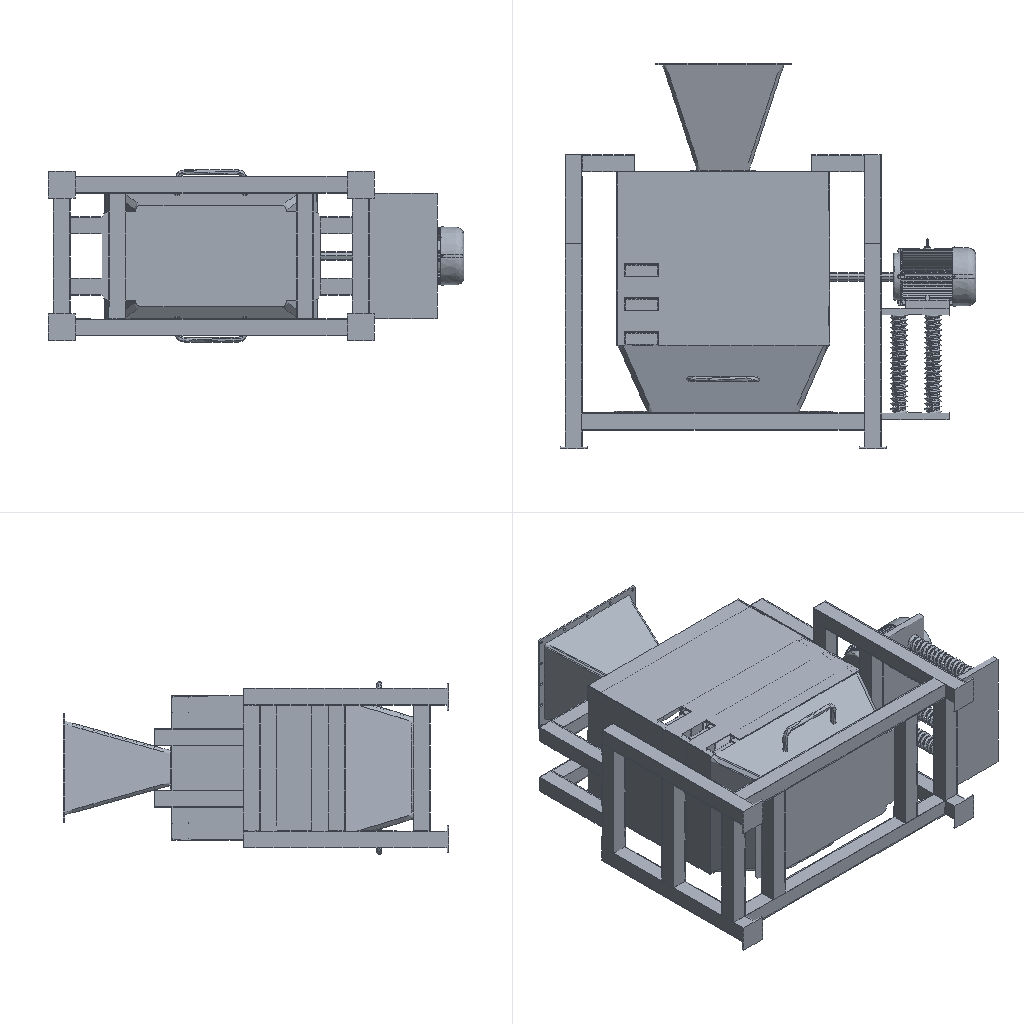Simulation study | ansys workbench
Set-up summary, first 221 of 611 lines:
category,name,step,type,value,unit,region
solver,ansys_mapdl
solver,version,,,21.2
solver,version,,,21.2
solver,version,,,21.2
solver,version,,,21.2
units,MPA,,stated
analysis,deck1,,modal,modal
load_step,requested,,,2
analysis,nlgeom,,,False
mesh,nodes,,,0
mesh,elements,,,0
load,load commands in deck,,count,0
bc,support commands in deck,,count,0
analysis,deck2,,static,static
load_step,requested,,,1
analysis,nlgeom,,,False
mesh,nodes,,,125678
mesh,elements,,,54949
element_type,ANSYS 187 (type 1),,solid,4190
element_type,ANSYS 186 (type 2),,solid,112
element_type,ANSYS 186 (type 3),,solid,154
element_type,ANSYS 186 (type 4),,solid,99
element_type,ANSYS 186 (type 5),,solid,109
element_type,ANSYS 186 (type 6),,solid,80
element_type,ANSYS 186 (type 7),,solid,144
element_type,ANSYS 186 (type 8),,solid,96
element_type,ANSYS 186 (type 9),,solid,96
element_type,ANSYS 186 (type 10),,solid,96
element_type,ANSYS 186 (type 11),,solid,132
element_type,ANSYS 186 (type 12),,solid,96
element_type,ANSYS 186 (type 13),,solid,132
element_type,ANSYS 187 (type 14),,solid,3160
element_type,ANSYS 186 (type 15),,solid,96
element_type,ANSYS 186 (type 16),,solid,96
element_type,ANSYS 186 (type 17),,solid,96
element_type,ANSYS 186 (type 18),,solid,88
element_type,ANSYS 186 (type 19),,solid,88
element_type,ANSYS 186 (type 20),,solid,88
element_type,ANSYS 186 (type 21),,solid,506
element_type,ANSYS 186 (type 22),,solid,80
element_type,ANSYS 186 (type 23),,solid,80
element_type,ANSYS 186 (type 24),,solid,80
element_type,ANSYS 186 (type 25),,solid,80
element_type,ANSYS 186 (type 26),,solid,80
element_type,ANSYS 187 (type 27),,solid,574
element_type,ANSYS 186 (type 28),,solid,45
element_type,ANSYS 186 (type 29),,solid,45
element_type,ANSYS 186 (type 30),,solid,20
element_type,ANSYS 186 (type 31),,solid,20
element_type,ANSYS 186 (type 32),,solid,20
element_type,ANSYS 186 (type 33),,solid,20
element_type,ANSYS 186 (type 34),,solid,20
element_type,ANSYS 186 (type 35),,solid,20
element_type,ANSYS 186 (type 36),,solid,160
element_type,ANSYS 186 (type 37),,solid,160
element_type,ANSYS 186 (type 38),,solid,160
element_type,ANSYS 186 (type 39),,solid,160
element_type,ANSYS 186 (type 40),,solid,160
element_type,ANSYS 186 (type 41),,solid,160
element_type,ANSYS 186 (type 42),,solid,160
element_type,ANSYS 186 (type 43),,solid,160
element_type,ANSYS 187 (type 44),,solid,19818
element_type,ANSYS 186 (type 45),,solid,144
element_type,ANSYS 186 (type 46),,solid,144
element_type,ANSYS 186 (type 47),,solid,144
element_type,ANSYS 186 (type 48),,solid,144
element_type,ANSYS 187 (type 49),,solid,1310
element_type,ANSYS 187 (type 50),,solid,1347
element_type,ANSYS 187 (type 51),,solid,1310
element_type,ANSYS 187 (type 52),,solid,1347
element_type,ANSYS 186 (type 53),,solid,128
element_type,ANSYS 186 (type 54),,solid,128
element_type,ANSYS 186 (type 55),,solid,128
element_type,ANSYS 186 (type 56),,solid,128
element_type,ANSYS 186 (type 57),,solid,192
element_type,ANSYS 186 (type 58),,solid,192
element_type,ANSYS 186 (type 59),,solid,192
element_type,ANSYS 186 (type 60),,solid,192
element_type,ANSYS 187 (type 61),,solid,1312
element_type,ANSYS 187 (type 62),,solid,1313
element_type,ANSYS 187 (type 63),,solid,1326
element_type,ANSYS 186 (type 64),,solid,36
element_type,ANSYS 186 (type 65),,solid,36
element_type,ANSYS 186 (type 66),,solid,36
element_type,ANSYS 186 (type 67),,solid,36
element_type,ANSYS 186 (type 68),,solid,56
element_type,ANSYS 186 (type 69),,solid,52
element_type,ANSYS 174 (type 70),,contact,70
element_type,ANSYS 170 (type 71),,target,70
element_type,ANSYS 174 (type 72),,contact,59
element_type,ANSYS 170 (type 73),,target,59
element_type,ANSYS 174 (type 74),,contact,64
element_type,ANSYS 170 (type 75),,target,64
element_type,ANSYS 174 (type 76),,contact,64
element_type,ANSYS 170 (type 77),,target,64
element_type,ANSYS 174 (type 78),,contact,254
element_type,ANSYS 170 (type 79),,target,254
element_type,ANSYS 174 (type 80),,contact,254
element_type,ANSYS 170 (type 81),,target,254
element_type,ANSYS 174 (type 82),,contact,14
element_type,ANSYS 170 (type 83),,target,14
element_type,ANSYS 174 (type 84),,contact,14
element_type,ANSYS 170 (type 85),,target,14
element_type,ANSYS 174 (type 86),,contact,32
element_type,ANSYS 170 (type 87),,target,32
element_type,ANSYS 174 (type 88),,contact,20
element_type,ANSYS 170 (type 89),,target,20
element_type,ANSYS 174 (type 90),,contact,17
element_type,ANSYS 170 (type 91),,target,17
element_type,ANSYS 174 (type 92),,contact,17
element_type,ANSYS 170 (type 93),,target,17
element_type,ANSYS 174 (type 94),,contact,20
element_type,ANSYS 170 (type 95),,target,20
element_type,ANSYS 174 (type 96),,contact,20
element_type,ANSYS 170 (type 97),,target,20
element_type,ANSYS 174 (type 98),,contact,19
element_type,ANSYS 170 (type 99),,target,19
element_type,ANSYS 174 (type 100),,contact,19
element_type,ANSYS 170 (type 101),,target,19
element_type,ANSYS 174 (type 102),,contact,46
element_type,ANSYS 170 (type 103),,target,46
element_type,ANSYS 174 (type 104),,contact,35
element_type,ANSYS 170 (type 105),,target,35
element_type,ANSYS 174 (type 106),,contact,46
element_type,ANSYS 170 (type 107),,target,46
element_type,ANSYS 174 (type 108),,contact,46
element_type,ANSYS 170 (type 109),,target,46
element_type,ANSYS 174 (type 110),,contact,9
element_type,ANSYS 170 (type 111),,target,9
element_type,ANSYS 174 (type 112),,contact,10
element_type,ANSYS 170 (type 113),,target,10
element_type,ANSYS 174 (type 114),,contact,10
element_type,ANSYS 170 (type 115),,target,10
element_type,ANSYS 174 (type 116),,contact,9
element_type,ANSYS 170 (type 117),,target,9
element_type,ANSYS 174 (type 118),,contact,10
element_type,ANSYS 170 (type 119),,target,10
element_type,ANSYS 174 (type 120),,contact,18
element_type,ANSYS 170 (type 121),,target,18
element_type,ANSYS 174 (type 122),,contact,2
element_type,ANSYS 170 (type 123),,target,2
element_type,ANSYS 174 (type 124),,contact,2
element_type,ANSYS 170 (type 125),,target,2
element_type,ANSYS 174 (type 126),,contact,3
element_type,ANSYS 170 (type 127),,target,3
element_type,ANSYS 174 (type 128),,contact,2
element_type,ANSYS 170 (type 129),,target,2
element_type,ANSYS 174 (type 130),,contact,2
element_type,ANSYS 170 (type 131),,target,2
element_type,ANSYS 174 (type 132),,contact,3
element_type,ANSYS 170 (type 133),,target,3
element_type,ANSYS 174 (type 134),,contact,25
element_type,ANSYS 170 (type 135),,target,25
element_type,ANSYS 174 (type 136),,contact,19
element_type,ANSYS 170 (type 137),,target,19
element_type,ANSYS 174 (type 138),,contact,46
element_type,ANSYS 170 (type 139),,target,46
element_type,ANSYS 174 (type 140),,contact,34
element_type,ANSYS 170 (type 141),,target,34
element_type,ANSYS 174 (type 142),,contact,45
element_type,ANSYS 170 (type 143),,target,45
element_type,ANSYS 174 (type 144),,contact,44
element_type,ANSYS 170 (type 145),,target,44
element_type,ANSYS 174 (type 146),,contact,12
element_type,ANSYS 170 (type 147),,target,12
element_type,ANSYS 174 (type 148),,contact,13
element_type,ANSYS 170 (type 149),,target,13
element_type,ANSYS 174 (type 150),,contact,15
element_type,ANSYS 170 (type 151),,target,15
element_type,ANSYS 174 (type 152),,contact,9
element_type,ANSYS 170 (type 153),,target,9
element_type,ANSYS 174 (type 154),,contact,10
element_type,ANSYS 170 (type 155),,target,10
element_type,ANSYS 174 (type 156),,contact,18
element_type,ANSYS 170 (type 157),,target,18
element_type,ANSYS 174 (type 158),,contact,5
element_type,ANSYS 170 (type 159),,target,5
element_type,ANSYS 174 (type 160),,contact,4
element_type,ANSYS 170 (type 161),,target,4
element_type,ANSYS 174 (type 162),,contact,5
element_type,ANSYS 170 (type 163),,target,5
element_type,ANSYS 174 (type 164),,contact,2
element_type,ANSYS 170 (type 165),,target,2
element_type,ANSYS 174 (type 166),,contact,2
element_type,ANSYS 170 (type 167),,target,2
element_type,ANSYS 174 (type 168),,contact,3
element_type,ANSYS 170 (type 169),,target,3
element_type,ANSYS 174 (type 170),,contact,12
element_type,ANSYS 170 (type 171),,target,12
element_type,ANSYS 174 (type 172),,contact,12
element_type,ANSYS 170 (type 173),,target,12
element_type,ANSYS 174 (type 174),,contact,28
element_type,ANSYS 170 (type 175),,target,28
element_type,ANSYS 174 (type 176),,contact,36
element_type,ANSYS 170 (type 177),,target,36
element_type,ANSYS 174 (type 178),,contact,36
element_type,ANSYS 170 (type 179),,target,36
element_type,ANSYS 174 (type 180),,contact,28
element_type,ANSYS 170 (type 181),,target,28
element_type,ANSYS 174 (type 182),,contact,28
element_type,ANSYS 170 (type 183),,target,28
element_type,ANSYS 174 (type 184),,contact,28
element_type,ANSYS 170 (type 185),,target,28
element_type,ANSYS 174 (type 186),,contact,52
element_type,ANSYS 170 (type 187),,target,52
element_type,ANSYS 174 (type 188),,contact,14
element_type,ANSYS 170 (type 189),,target,14
element_type,ANSYS 174 (type 190),,contact,14
element_type,ANSYS 170 (type 191),,target,14
element_type,ANSYS 174 (type 192),,contact,12
element_type,ANSYS 170 (type 193),,target,12
element_type,ANSYS 174 (type 194),,contact,12
element_type,ANSYS 170 (type 195),,target,12
element_type,ANSYS 174 (type 196),,contact,33
element_type,ANSYS 170 (type 197),,target,33
element_type,ANSYS 174 (type 198),,contact,45
element_type,ANSYS 170 (type 199),,target,45
element_type,ANSYS 174 (type 200),,contact,109
element_type,ANSYS 170 (type 201),,target,109
element_type,ANSYS 174 (type 202),,contact,28
Results summary:
result,analysis,,,modal
result,last_loadstep,,,1
result,primary field,,,displacement
result,analysis,,,static
result,last_loadstep,,,1
result,primary field,,,displacement
result,mass,,,0.09057,"NMM: mm, ton, N, s, mV, mA, degC"
result,analysis,,,static
result,last_loadstep,,,1
result,primary field,,,displacement
result,reaction total,1,FX,4.4e-05,N
result,reaction total,1,FY,21656.525,N
result,reaction total,1,FZ,5.6e-05,N
result,mass,,,0.07835,"NMM: mm, ton, N, s, mV, mA, degC"
result,analysis,,,static
result,last_loadstep,,,1
result,primary field,,,displacement
result,reaction total,1,FX,4.4e-05,N
result,reaction total,1,FY,21656.525,N
result,reaction total,1,FZ,5.6e-05,N
result,mass,,,0.1689,"NMM: mm, ton, N, s, mV, mA, degC"